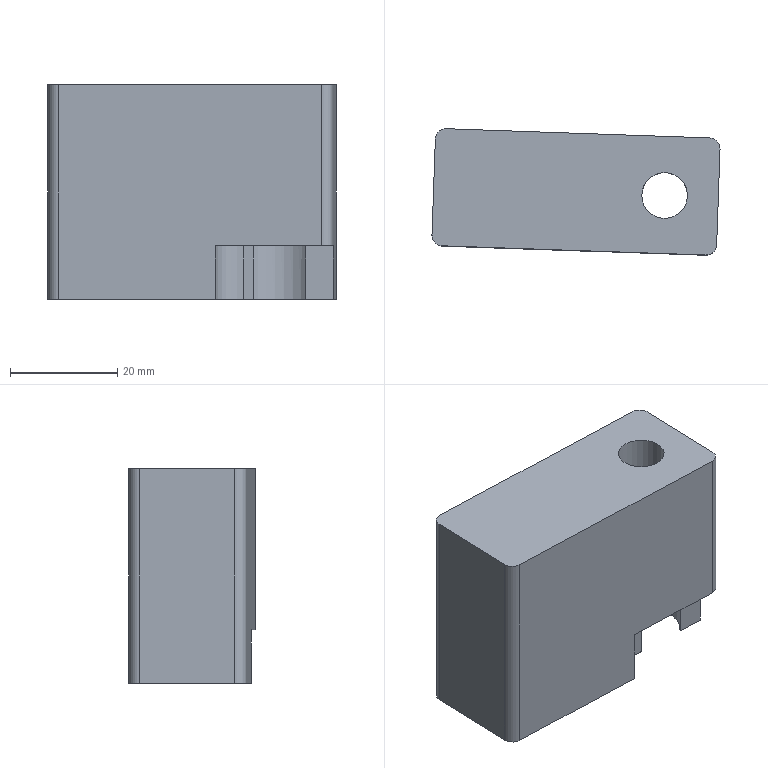Part | NX | features PS-34 2 | 1 solid | 18 faces | box 53.591 x 23.499 x 40 mm | volume 40103 mm3 | plane 11 | cylinder 7 | commonest cylinder face diameters 4 x4 8.5 x1 10 x1 14.5 x1
STEP:
#1=CARTESIAN_POINT('',(3532.617,-894.43,870.698));
#2=VERTEX_POINT('',#1);
#3=CARTESIAN_POINT('',(3530.744,-894.365,870.698));
#4=VERTEX_POINT('',#3);
#5=CARTESIAN_POINT('',(3542.677,-894.781,870.698));
#6=DIRECTION('',(-0.9994,0.0349,-0.000000001));
#7=VECTOR('',#6,1000.);
#8=LINE('',#5,#7);
#9=EDGE_CURVE('',#2,#4,#8,.T.);
#10=ORIENTED_EDGE('',*,*,#9,.T.);
#11=CARTESIAN_POINT('',(3530.744,-894.365,860.716));
#12=VERTEX_POINT('',#11);
#13=CARTESIAN_POINT('',(3530.744,-894.365,845.698));
#14=DIRECTION('',(-0.000000001,0.,1.));
#15=VECTOR('',#14,1000.);
#16=LINE('',#13,#15);
#17=EDGE_CURVE('',#4,#12,#16,.F.);
#18=ORIENTED_EDGE('',*,*,#17,.T.);
#19=CARTESIAN_POINT('',(3532.617,-894.43,860.716));
#20=VERTEX_POINT('',#19);
#21=CARTESIAN_POINT('',(3551.671,-895.095,860.716));
#22=DIRECTION('',(0.9994,-0.0349,0.));
#23=VECTOR('',#22,1000.);
#24=LINE('',#21,#23);
#25=EDGE_CURVE('',#12,#20,#24,.T.);
#26=ORIENTED_EDGE('',*,*,#25,.T.);
#27=CARTESIAN_POINT('',(3532.617,-894.43,870.698));
#28=CARTESIAN_POINT('',(3532.617,-894.43,867.371));
#29=CARTESIAN_POINT('',(3532.617,-894.43,864.044));
#30=CARTESIAN_POINT('',(3532.617,-894.43,860.716));
#31=B_SPLINE_CURVE_WITH_KNOTS('',3,(#27,#28,#29,#30),.UNSPECIFIED.,.F.,.F.,(4,4),(0.0000002,0.009982),.UNSPECIFIED.);
#32=EDGE_CURVE('',#2,#20,#31,.T.);
#33=ORIENTED_EDGE('',*,*,#32,.F.);
#34=EDGE_LOOP('',(#10,#18,#26,#33));
#35=FACE_BOUND('',#34,.T.);
#36=CARTESIAN_POINT('',(3542.677,-894.781,845.698));
#37=DIRECTION('',(0.0349,0.9994,0.));
#38=DIRECTION('',(0.9994,-0.0349,0.));
#39=AXIS2_PLACEMENT_3D('',#36,#37,#38);
#40=PLANE('',#39);
#41=ADVANCED_FACE('',(#35),#40,.F.);
#42=CARTESIAN_POINT('',(3525.557,-899.644,860.716));
#43=VERTEX_POINT('',#42);
#44=CARTESIAN_POINT('',(3525.557,-899.644,870.698));
#45=VERTEX_POINT('',#44);
#46=CARTESIAN_POINT('',(3525.557,-899.644,845.698));
#47=DIRECTION('',(-0.000000001,0.,1.));
#48=VECTOR('',#47,1000.);
#49=LINE('',#46,#48);
#50=EDGE_CURVE('',#43,#45,#49,.T.);
#51=ORIENTED_EDGE('',*,*,#50,.T.);
#52=CARTESIAN_POINT('',(3545.32,-900.334,870.698));
#53=VERTEX_POINT('',#52);
#54=CARTESIAN_POINT('',(3529.824,-899.793,870.698));
#55=DIRECTION('',(-0.9994,0.0349,-0.000000001));
#56=VECTOR('',#55,1000.);
#57=LINE('',#54,#56);
#58=EDGE_CURVE('',#53,#45,#57,.T.);
#59=ORIENTED_EDGE('',*,*,#58,.F.);
#60=CARTESIAN_POINT('',(3545.32,-900.334,900.716));
#61=VERTEX_POINT('',#60);
#62=CARTESIAN_POINT('',(3545.32,-900.334,860.716));
#63=DIRECTION('',(0.,0.,-1.));
#64=VECTOR('',#63,1000.);
#65=LINE('',#62,#64);
#66=EDGE_CURVE('',#61,#53,#65,.T.);
#67=ORIENTED_EDGE('',*,*,#66,.F.);
#68=CARTESIAN_POINT('',(3496.35,-898.624,900.716));
#69=VERTEX_POINT('',#68);
#70=CARTESIAN_POINT('',(3551.481,-900.549,900.716));
#71=DIRECTION('',(0.9994,-0.0349,0.));
#72=VECTOR('',#71,1000.);
#73=LINE('',#70,#72);
#74=EDGE_CURVE('',#69,#61,#73,.T.);
#75=ORIENTED_EDGE('',*,*,#74,.F.);
#76=CARTESIAN_POINT('',(3496.35,-898.624,860.716));
#77=VERTEX_POINT('',#76);
#78=CARTESIAN_POINT('',(3496.35,-898.624,900.716));
#79=DIRECTION('',(0.,0.,1.));
#80=VECTOR('',#79,1000.);
#81=LINE('',#78,#80);
#82=EDGE_CURVE('',#77,#69,#81,.T.);
#83=ORIENTED_EDGE('',*,*,#82,.F.);
#84=CARTESIAN_POINT('',(3551.481,-900.549,860.716));
#85=DIRECTION('',(0.9994,-0.0349,0.));
#86=VECTOR('',#85,1000.);
#87=LINE('',#84,#86);
#88=EDGE_CURVE('',#77,#43,#87,.T.);
#89=ORIENTED_EDGE('',*,*,#88,.T.);
#90=EDGE_LOOP('',(#51,#59,#67,#75,#83,#89));
#91=FACE_BOUND('',#90,.T.);
#92=CARTESIAN_POINT('',(3551.481,-900.549,950.716));
#93=DIRECTION('',(0.0349,0.9994,0.));
#94=DIRECTION('',(-0.9994,0.0349,0.));
#95=AXIS2_PLACEMENT_3D('',#92,#93,#94);
#96=PLANE('',#95);
#97=ADVANCED_FACE('',(#91),#96,.F.);
#98=CARTESIAN_POINT('',(3547.509,-894.95,870.698));
#99=VERTEX_POINT('',#98);
#100=CARTESIAN_POINT('',(3547.509,-894.95,860.716));
#101=VERTEX_POINT('',#100);
#102=CARTESIAN_POINT('',(3547.509,-894.95,860.716));
#103=DIRECTION('',(0.,0.,-1.));
#104=VECTOR('',#103,1000.);
#105=LINE('',#102,#104);
#106=EDGE_CURVE('',#99,#101,#105,.T.);
#107=ORIENTED_EDGE('',*,*,#106,.T.);
#108=CARTESIAN_POINT('',(3548.009,-880.616,860.716));
#109=VERTEX_POINT('',#108);
#110=CARTESIAN_POINT('',(3548.184,-875.619,860.716));
#111=DIRECTION('',(-0.0349,-0.9994,0.));
#112=VECTOR('',#111,1000.);
#113=LINE('',#110,#112);
#114=EDGE_CURVE('',#109,#101,#113,.T.);
#115=ORIENTED_EDGE('',*,*,#114,.F.);
#116=CARTESIAN_POINT('',(3548.009,-880.616,900.716));
#117=VERTEX_POINT('',#116);
#118=CARTESIAN_POINT('',(3548.009,-880.616,860.716));
#119=DIRECTION('',(0.,0.,-1.));
#120=VECTOR('',#119,1000.);
#121=LINE('',#118,#120);
#122=EDGE_CURVE('',#117,#109,#121,.T.);
#123=ORIENTED_EDGE('',*,*,#122,.F.);
#124=CARTESIAN_POINT('',(3547.388,-898.405,900.716));
#125=VERTEX_POINT('',#124);
#126=CARTESIAN_POINT('',(3548.184,-875.619,900.716));
#127=DIRECTION('',(-0.0349,-0.9994,0.));
#128=VECTOR('',#127,1000.);
#129=LINE('',#126,#128);
#130=EDGE_CURVE('',#117,#125,#129,.T.);
#131=ORIENTED_EDGE('',*,*,#130,.T.);
#132=CARTESIAN_POINT('',(3547.388,-898.405,870.698));
#133=VERTEX_POINT('',#132);
#134=CARTESIAN_POINT('',(3547.388,-898.405,900.716));
#135=DIRECTION('',(0.,0.,-1.));
#136=VECTOR('',#135,1000.);
#137=LINE('',#134,#136);
#138=EDGE_CURVE('',#133,#125,#137,.F.);
#139=ORIENTED_EDGE('',*,*,#138,.F.);
#140=CARTESIAN_POINT('',(3548.184,-875.619,870.698));
#141=DIRECTION('',(0.0349,0.9994,0.));
#142=VECTOR('',#141,1000.);
#143=LINE('',#140,#142);
#144=EDGE_CURVE('',#133,#99,#143,.T.);
#145=ORIENTED_EDGE('',*,*,#144,.T.);
#146=EDGE_LOOP('',(#107,#115,#123,#131,#139,#145));
#147=FACE_BOUND('',#146,.T.);
#148=CARTESIAN_POINT('',(3548.184,-875.619,860.716));
#149=DIRECTION('',(0.9994,-0.0349,0.));
#150=DIRECTION('',(-0.0349,-0.9994,0.));
#151=AXIS2_PLACEMENT_3D('',#148,#149,#150);
#152=PLANE('',#151);
#153=ADVANCED_FACE('',(#147),#152,.T.);
#154=CARTESIAN_POINT('',(3541.951,-889.261,900.716));
#155=VERTEX_POINT('',#154);
#156=CARTESIAN_POINT('',(3537.701,-889.261,900.716));
#157=DIRECTION('',(0.,0.,-1.));
#158=DIRECTION('',(1.,0.,0.));
#159=AXIS2_PLACEMENT_3D('',#156,#157,#158);
#160=CIRCLE('',#159,4.25);
#161=EDGE_CURVE('',#155,#155,#160,.T.);
#162=ORIENTED_EDGE('',*,*,#161,.T.);
#163=EDGE_LOOP('',(#162));
#164=FACE_BOUND('',#163,.T.);
#165=CARTESIAN_POINT('',(3495.042,-878.766,900.716));
#166=VERTEX_POINT('',#165);
#167=CARTESIAN_POINT('',(3494.421,-896.556,900.716));
#168=VERTEX_POINT('',#167);
#169=CARTESIAN_POINT('',(3495.216,-873.77,900.716));
#170=DIRECTION('',(-0.0349,-0.9994,0.));
#171=VECTOR('',#170,1000.);
#172=LINE('',#169,#171);
#173=EDGE_CURVE('',#166,#168,#172,.T.);
#174=ORIENTED_EDGE('',*,*,#173,.T.);
#175=CARTESIAN_POINT('',(3496.419,-896.625,900.716));
#176=DIRECTION('',(0.,0.,-1.));
#177=DIRECTION('',(1.,0.,0.));
#178=AXIS2_PLACEMENT_3D('',#175,#176,#177);
#179=CIRCLE('',#178,2.);
#180=EDGE_CURVE('',#69,#168,#179,.T.);
#181=ORIENTED_EDGE('',*,*,#180,.F.);
#182=ORIENTED_EDGE('',*,*,#74,.T.);
#183=CARTESIAN_POINT('',(3545.39,-898.335,900.716));
#184=DIRECTION('',(0.,0.,-1.));
#185=DIRECTION('',(1.,0.,0.));
#186=AXIS2_PLACEMENT_3D('',#183,#184,#185);
#187=CIRCLE('',#186,2.);
#188=EDGE_CURVE('',#125,#61,#187,.T.);
#189=ORIENTED_EDGE('',*,*,#188,.F.);
#190=ORIENTED_EDGE('',*,*,#130,.F.);
#191=CARTESIAN_POINT('',(3546.08,-878.547,900.716));
#192=VERTEX_POINT('',#191);
#193=CARTESIAN_POINT('',(3546.011,-880.546,900.716));
#194=DIRECTION('',(0.,0.,-1.));
#195=DIRECTION('',(1.,0.,0.));
#196=AXIS2_PLACEMENT_3D('',#193,#194,#195);
#197=CIRCLE('',#196,2.);
#198=EDGE_CURVE('',#192,#117,#197,.T.);
#199=ORIENTED_EDGE('',*,*,#198,.F.);
#200=CARTESIAN_POINT('',(3497.11,-876.837,900.716));
#201=VERTEX_POINT('',#200);
#202=CARTESIAN_POINT('',(3552.241,-878.762,900.716));
#203=DIRECTION('',(0.9994,-0.0349,0.));
#204=VECTOR('',#203,1000.);
#205=LINE('',#202,#204);
#206=EDGE_CURVE('',#201,#192,#205,.T.);
#207=ORIENTED_EDGE('',*,*,#206,.F.);
#208=CARTESIAN_POINT('',(3497.041,-878.836,900.716));
#209=DIRECTION('',(0.,0.,-1.));
#210=DIRECTION('',(1.,0.,0.));
#211=AXIS2_PLACEMENT_3D('',#208,#209,#210);
#212=CIRCLE('',#211,2.);
#213=EDGE_CURVE('',#166,#201,#212,.T.);
#214=ORIENTED_EDGE('',*,*,#213,.F.);
#215=EDGE_LOOP('',(#174,#181,#182,#189,#190,#199,#207,#214));
#216=FACE_BOUND('',#215,.T.);
#217=CARTESIAN_POINT('',(3552.346,-875.764,900.716));
#218=DIRECTION('',(0.,0.,1.));
#219=DIRECTION('',(1.,0.,0.));
#220=AXIS2_PLACEMENT_3D('',#217,#218,#219);
#221=PLANE('',#220);
#222=ADVANCED_FACE('',(#164,#216),#221,.T.);
#223=CARTESIAN_POINT('',(3495.042,-878.766,860.716));
#224=VERTEX_POINT('',#223);
#225=CARTESIAN_POINT('',(3494.421,-896.556,860.716));
#226=VERTEX_POINT('',#225);
#227=CARTESIAN_POINT('',(3495.216,-873.77,860.716));
#228=DIRECTION('',(-0.0349,-0.9994,0.));
#229=VECTOR('',#228,1000.);
#230=LINE('',#227,#229);
#231=EDGE_CURVE('',#224,#226,#230,.T.);
#232=ORIENTED_EDGE('',*,*,#231,.T.);
#233=CARTESIAN_POINT('',(3494.421,-896.556,860.716));
#234=DIRECTION('',(0.,0.,1.));
#235=VECTOR('',#234,1000.);
#236=LINE('',#233,#235);
#237=EDGE_CURVE('',#168,#226,#236,.F.);
#238=ORIENTED_EDGE('',*,*,#237,.F.);
#239=ORIENTED_EDGE('',*,*,#173,.F.);
#240=CARTESIAN_POINT('',(3495.042,-878.766,950.716));
#241=DIRECTION('',(0.,0.,-1.));
#242=VECTOR('',#241,1000.);
#243=LINE('',#240,#242);
#244=EDGE_CURVE('',#224,#166,#243,.F.);
#245=ORIENTED_EDGE('',*,*,#244,.F.);
#246=EDGE_LOOP('',(#232,#238,#239,#245));
#247=FACE_BOUND('',#246,.T.);
#248=CARTESIAN_POINT('',(3495.216,-873.77,950.716));
#249=DIRECTION('',(-0.9994,0.0349,0.));
#250=DIRECTION('',(0.0349,0.9994,0.));
#251=AXIS2_PLACEMENT_3D('',#248,#249,#250);
#252=PLANE('',#251);
#253=ADVANCED_FACE('',(#247),#252,.T.);
#254=ORIENTED_EDGE('',*,*,#25,.F.);
#255=CARTESIAN_POINT('',(3525.573,-899.187,860.716));
#256=VERTEX_POINT('',#255);
#257=CARTESIAN_POINT('',(3530.57,-899.361,860.716));
#258=DIRECTION('',(0.,0.,-1.));
#259=DIRECTION('',(1.,0.,0.));
#260=AXIS2_PLACEMENT_3D('',#257,#258,#259);
#261=CIRCLE('',#260,5.);
#262=EDGE_CURVE('',#12,#256,#261,.F.);
#263=ORIENTED_EDGE('',*,*,#262,.T.);
#264=CARTESIAN_POINT('',(3526.422,-874.859,860.716));
#265=DIRECTION('',(-0.0349,-0.9994,0.));
#266=VECTOR('',#265,1000.);
#267=LINE('',#264,#266);
#268=EDGE_CURVE('',#256,#43,#267,.T.);
#269=ORIENTED_EDGE('',*,*,#268,.T.);
#270=ORIENTED_EDGE('',*,*,#88,.F.);
#271=CARTESIAN_POINT('',(3496.419,-896.625,860.716));
#272=DIRECTION('',(0.,0.,-1.));
#273=DIRECTION('',(1.,0.,0.));
#274=AXIS2_PLACEMENT_3D('',#271,#272,#273);
#275=CIRCLE('',#274,2.);
#276=EDGE_CURVE('',#226,#77,#275,.F.);
#277=ORIENTED_EDGE('',*,*,#276,.F.);
#278=ORIENTED_EDGE('',*,*,#231,.F.);
#279=CARTESIAN_POINT('',(3497.11,-876.837,860.716));
#280=VERTEX_POINT('',#279);
#281=CARTESIAN_POINT('',(3497.041,-878.836,860.716));
#282=DIRECTION('',(0.,0.,-1.));
#283=DIRECTION('',(1.,0.,0.));
#284=AXIS2_PLACEMENT_3D('',#281,#282,#283);
#285=CIRCLE('',#284,2.);
#286=EDGE_CURVE('',#280,#224,#285,.F.);
#287=ORIENTED_EDGE('',*,*,#286,.F.);
#288=CARTESIAN_POINT('',(3546.08,-878.547,860.716));
#289=VERTEX_POINT('',#288);
#290=CARTESIAN_POINT('',(3552.241,-878.762,860.716));
#291=DIRECTION('',(0.9994,-0.0349,0.));
#292=VECTOR('',#291,1000.);
#293=LINE('',#290,#292);
#294=EDGE_CURVE('',#289,#280,#293,.F.);
#295=ORIENTED_EDGE('',*,*,#294,.F.);
#296=CARTESIAN_POINT('',(3546.011,-880.546,860.716));
#297=DIRECTION('',(0.,0.,-1.));
#298=DIRECTION('',(1.,0.,0.));
#299=AXIS2_PLACEMENT_3D('',#296,#297,#298);
#300=CIRCLE('',#299,2.);
#301=EDGE_CURVE('',#109,#289,#300,.F.);
#302=ORIENTED_EDGE('',*,*,#301,.F.);
#303=ORIENTED_EDGE('',*,*,#114,.T.);
#304=CARTESIAN_POINT('',(3542.413,-894.772,860.716));
#305=VERTEX_POINT('',#304);
#306=CARTESIAN_POINT('',(3551.671,-895.095,860.716));
#307=DIRECTION('',(0.9994,-0.0349,0.));
#308=VECTOR('',#307,1000.);
#309=LINE('',#306,#308);
#310=EDGE_CURVE('',#305,#101,#309,.T.);
#311=ORIENTED_EDGE('',*,*,#310,.F.);
#312=CARTESIAN_POINT('',(3537.701,-889.261,860.716));
#313=DIRECTION('',(0.,0.,-1.));
#314=DIRECTION('',(1.,0.,0.));
#315=AXIS2_PLACEMENT_3D('',#312,#313,#314);
#316=CIRCLE('',#315,7.25);
#317=EDGE_CURVE('',#20,#305,#316,.T.);
#318=ORIENTED_EDGE('',*,*,#317,.F.);
#319=EDGE_LOOP('',(#254,#263,#269,#270,#277,#278,#287,#295,#302,#303,#311,#318));
#320=FACE_BOUND('',#319,.T.);
#321=CARTESIAN_POINT('',(3552.346,-875.764,860.716));
#322=DIRECTION('',(0.,0.,1.));
#323=DIRECTION('',(1.,0.,0.));
#324=AXIS2_PLACEMENT_3D('',#321,#322,#323);
#325=PLANE('',#324);
#326=ADVANCED_FACE('',(#320),#325,.F.);
#327=ORIENTED_EDGE('',*,*,#206,.T.);
#328=CARTESIAN_POINT('',(3546.08,-878.547,880.716));
#329=DIRECTION('',(0.,0.,-1.));
#330=VECTOR('',#329,1000.);
#331=LINE('',#328,#330);
#332=EDGE_CURVE('',#289,#192,#331,.F.);
#333=ORIENTED_EDGE('',*,*,#332,.F.);
#334=ORIENTED_EDGE('',*,*,#294,.T.);
#335=CARTESIAN_POINT('',(3497.11,-876.837,880.716));
#336=DIRECTION('',(0.,0.,-1.));
#337=VECTOR('',#336,1000.);
#338=LINE('',#335,#337);
#339=EDGE_CURVE('',#201,#280,#338,.T.);
#340=ORIENTED_EDGE('',*,*,#339,.F.);
#341=EDGE_LOOP('',(#327,#333,#334,#340));
#342=FACE_BOUND('',#341,.T.);
#343=CARTESIAN_POINT('',(3514.1,-877.431,880.716));
#344=DIRECTION('',(0.0349,0.9994,0.));
#345=DIRECTION('',(0.9994,-0.0349,0.));
#346=AXIS2_PLACEMENT_3D('',#343,#344,#345);
#347=PLANE('',#346);
#348=ADVANCED_FACE('',(#342),#347,.T.);
#349=ORIENTED_EDGE('',*,*,#213,.T.);
#350=ORIENTED_EDGE('',*,*,#339,.T.);
#351=ORIENTED_EDGE('',*,*,#286,.T.);
#352=ORIENTED_EDGE('',*,*,#244,.T.);
#353=EDGE_LOOP('',(#349,#350,#351,#352));
#354=FACE_BOUND('',#353,.T.);
#355=CARTESIAN_POINT('',(3497.041,-878.836,880.716));
#356=DIRECTION('',(0.,0.,-1.));
#357=DIRECTION('',(-1.,0.,0.));
#358=AXIS2_PLACEMENT_3D('',#355,#356,#357);
#359=CYLINDRICAL_SURFACE('',#358,2.);
#360=ADVANCED_FACE('',(#354),#359,.T.);
#361=ORIENTED_EDGE('',*,*,#198,.T.);
#362=ORIENTED_EDGE('',*,*,#122,.T.);
#363=ORIENTED_EDGE('',*,*,#301,.T.);
#364=ORIENTED_EDGE('',*,*,#332,.T.);
#365=EDGE_LOOP('',(#361,#362,#363,#364));
#366=FACE_BOUND('',#365,.T.);
#367=CARTESIAN_POINT('',(3546.011,-880.546,860.716));
#368=DIRECTION('',(0.,0.,-1.));
#369=DIRECTION('',(-1.,0.,0.));
#370=AXIS2_PLACEMENT_3D('',#367,#368,#369);
#371=CYLINDRICAL_SURFACE('',#370,2.);
#372=ADVANCED_FACE('',(#366),#371,.T.);
#373=CARTESIAN_POINT('',(3545.39,-898.335,870.698));
#374=DIRECTION('',(0.000000001,0.,-1.));
#375=DIRECTION('',(1.,0.,0.000000001));
#376=AXIS2_PLACEMENT_3D('',#373,#374,#375);
#377=CIRCLE('',#376,2.);
#378=EDGE_CURVE('',#53,#133,#377,.F.);
#379=ORIENTED_EDGE('',*,*,#378,.T.);
#380=ORIENTED_EDGE('',*,*,#138,.T.);
#381=ORIENTED_EDGE('',*,*,#188,.T.);
#382=ORIENTED_EDGE('',*,*,#66,.T.);
#383=EDGE_LOOP('',(#379,#380,#381,#382));
#384=FACE_BOUND('',#383,.T.);
#385=CARTESIAN_POINT('',(3545.39,-898.335,950.716));
#386=DIRECTION('',(0.,0.,1.));
#387=DIRECTION('',(1.,0.,0.));
#388=AXIS2_PLACEMENT_3D('',#385,#386,#387);
#389=CYLINDRICAL_SURFACE('',#388,2.);
#390=ADVANCED_FACE('',(#384),#389,.T.);
#391=ORIENTED_EDGE('',*,*,#276,.T.);
#392=ORIENTED_EDGE('',*,*,#82,.T.);
#393=ORIENTED_EDGE('',*,*,#180,.T.);
#394=ORIENTED_EDGE('',*,*,#237,.T.);
#395=EDGE_LOOP('',(#391,#392,#393,#394));
#396=FACE_BOUND('',#395,.T.);
#397=CARTESIAN_POINT('',(3496.419,-896.625,950.716));
#398=DIRECTION('',(0.,0.,-1.));
#399=DIRECTION('',(-1.,0.,0.));
#400=AXIS2_PLACEMENT_3D('',#397,#398,#399);
#401=CYLINDRICAL_SURFACE('',#400,2.);
#402=ADVANCED_FACE('',(#396),#401,.T.);
#403=ORIENTED_EDGE('',*,*,#262,.F.);
#404=ORIENTED_EDGE('',*,*,#17,.F.);
#405=CARTESIAN_POINT('',(3525.573,-899.187,870.698));
#406=VERTEX_POINT('',#405);
#407=CARTESIAN_POINT('',(3530.57,-899.361,870.698));
#408=DIRECTION('',(0.000000001,0.,-1.));
#409=DIRECTION('',(1.,0.,0.000000001));
#410=AXIS2_PLACEMENT_3D('',#407,#408,#409);
#411=CIRCLE('',#410,5.);
#412=EDGE_CURVE('',#406,#4,#411,.T.);
#413=ORIENTED_EDGE('',*,*,#412,.F.);
#414=CARTESIAN_POINT('',(3525.573,-899.187,845.698));
#415=DIRECTION('',(-0.000000001,0.,1.));
#416=VECTOR('',#415,1000.);
#417=LINE('',#414,#416);
#418=EDGE_CURVE('',#406,#256,#417,.F.);
#419=ORIENTED_EDGE('',*,*,#418,.T.);
#420=EDGE_LOOP('',(#403,#404,#413,#419));
#421=FACE_BOUND('',#420,.T.);
#422=CARTESIAN_POINT('',(3530.57,-899.361,845.698));
#423=DIRECTION('',(-0.000000001,0.,1.));
#424=DIRECTION('',(1.,0.,0.000000001));
#425=AXIS2_PLACEMENT_3D('',#422,#423,#424);
#426=CYLINDRICAL_SURFACE('',#425,5.);
#427=ADVANCED_FACE('',(#421),#426,.F.);
#428=ORIENTED_EDGE('',*,*,#268,.F.);
#429=ORIENTED_EDGE('',*,*,#418,.F.);
#430=CARTESIAN_POINT('',(3525.258,-908.206,870.698));
#431=DIRECTION('',(0.0349,0.9994,0.));
#432=VECTOR('',#431,1000.);
#433=LINE('',#430,#432);
#434=EDGE_CURVE('',#45,#406,#433,.T.);
#435=ORIENTED_EDGE('',*,*,#434,.F.);
#436=ORIENTED_EDGE('',*,*,#50,.F.);
#437=EDGE_LOOP('',(#428,#429,#435,#436));
#438=FACE_BOUND('',#437,.T.);
#439=CARTESIAN_POINT('',(3525.258,-908.206,845.698));
#440=DIRECTION('',(0.9994,-0.0349,0.000000001));
#441=DIRECTION('',(-0.0349,-0.9994,0.));
#442=AXIS2_PLACEMENT_3D('',#439,#440,#441);
#443=PLANE('',#442);
#444=ADVANCED_FACE('',(#438),#443,.T.);
#445=ORIENTED_EDGE('',*,*,#310,.T.);
#446=ORIENTED_EDGE('',*,*,#106,.F.);
#447=CARTESIAN_POINT('',(3542.413,-894.772,870.698));
#448=VERTEX_POINT('',#447);
#449=CARTESIAN_POINT('',(3542.677,-894.781,870.698));
#450=DIRECTION('',(-0.9994,0.0349,-0.000000001));
#451=VECTOR('',#450,1000.);
#452=LINE('',#449,#451);
#453=EDGE_CURVE('',#99,#448,#452,.T.);
#454=ORIENTED_EDGE('',*,*,#453,.T.);
#455=CARTESIAN_POINT('',(3542.413,-894.772,860.716));
#456=CARTESIAN_POINT('',(3542.413,-894.772,864.044));
#457=CARTESIAN_POINT('',(3542.413,-894.772,867.371));
#458=CARTESIAN_POINT('',(3542.413,-894.772,870.698));
#459=B_SPLINE_CURVE_WITH_KNOTS('',3,(#455,#456,#457,#458),.UNSPECIFIED.,.F.,.F.,(4,4),(0.0000002,0.009982),.UNSPECIFIED.);
#460=EDGE_CURVE('',#305,#448,#459,.T.);
#461=ORIENTED_EDGE('',*,*,#460,.F.);
#462=EDGE_LOOP('',(#445,#446,#454,#461));
#463=FACE_BOUND('',#462,.T.);
#464=CARTESIAN_POINT('',(3542.677,-894.781,845.698));
#465=DIRECTION('',(0.0349,0.9994,0.));
#466=DIRECTION('',(0.9994,-0.0349,0.));
#467=AXIS2_PLACEMENT_3D('',#464,#465,#466);
#468=PLANE('',#467);
#469=ADVANCED_FACE('',(#463),#468,.F.);
#470=ORIENTED_EDGE('',*,*,#453,.F.);
#471=ORIENTED_EDGE('',*,*,#144,.F.);
#472=ORIENTED_EDGE('',*,*,#378,.F.);
#473=ORIENTED_EDGE('',*,*,#58,.T.);
#474=ORIENTED_EDGE('',*,*,#434,.T.);
#475=ORIENTED_EDGE('',*,*,#412,.T.);
#476=ORIENTED_EDGE('',*,*,#9,.F.);
#477=CARTESIAN_POINT('',(3537.701,-889.261,870.698));
#478=DIRECTION('',(0.000000001,0.,-1.));
#479=DIRECTION('',(1.,0.,0.000000001));
#480=AXIS2_PLACEMENT_3D('',#477,#478,#479);
#481=CIRCLE('',#480,7.25);
#482=EDGE_CURVE('',#448,#2,#481,.T.);
#483=ORIENTED_EDGE('',*,*,#482,.F.);
#484=EDGE_LOOP('',(#470,#471,#472,#473,#474,#475,#476,#483));
#485=FACE_BOUND('',#484,.T.);
#486=CARTESIAN_POINT('',(3529.525,-908.355,870.698));
#487=DIRECTION('',(-0.000000001,0.,1.));
#488=DIRECTION('',(1.,0.,0.000000001));
#489=AXIS2_PLACEMENT_3D('',#486,#487,#488);
#490=PLANE('',#489);
#491=ADVANCED_FACE('',(#485),#490,.F.);
#492=CARTESIAN_POINT('',(3530.451,-889.261,885.716));
#493=VERTEX_POINT('',#492);
#494=CARTESIAN_POINT('',(3537.701,-889.261,885.716));
#495=DIRECTION('',(0.,0.,1.));
#496=DIRECTION('',(-1.,0.,0.));
#497=AXIS2_PLACEMENT_3D('',#494,#495,#496);
#498=CIRCLE('',#497,7.25);
#499=EDGE_CURVE('',#493,#493,#498,.F.);
#500=ORIENTED_EDGE('',*,*,#499,.F.);
#501=EDGE_LOOP('',(#500));
#502=FACE_BOUND('',#501,.T.);
#503=ORIENTED_EDGE('',*,*,#32,.T.);
#504=ORIENTED_EDGE('',*,*,#317,.T.);
#505=ORIENTED_EDGE('',*,*,#460,.T.);
#506=ORIENTED_EDGE('',*,*,#482,.T.);
#507=EDGE_LOOP('',(#503,#504,#505,#506));
#508=FACE_BOUND('',#507,.T.);
#509=CARTESIAN_POINT('',(3537.701,-889.261,875.716));
#510=DIRECTION('',(0.,0.,-1.));
#511=DIRECTION('',(-1.,0.,0.));
#512=AXIS2_PLACEMENT_3D('',#509,#510,#511);
#513=CYLINDRICAL_SURFACE('',#512,7.25);
#514=ADVANCED_FACE('',(#502,#508),#513,.F.);
#515=ORIENTED_EDGE('',*,*,#161,.F.);
#516=EDGE_LOOP('',(#515));
#517=FACE_BOUND('',#516,.T.);
#518=CARTESIAN_POINT('',(3533.451,-889.261,885.716));
#519=VERTEX_POINT('',#518);
#520=CARTESIAN_POINT('',(3537.701,-889.261,885.716));
#521=DIRECTION('',(0.,0.,1.));
#522=DIRECTION('',(-1.,0.,0.));
#523=AXIS2_PLACEMENT_3D('',#520,#521,#522);
#524=CIRCLE('',#523,4.25);
#525=EDGE_CURVE('',#519,#519,#524,.T.);
#526=ORIENTED_EDGE('',*,*,#525,.F.);
#527=EDGE_LOOP('',(#526));
#528=FACE_BOUND('',#527,.T.);
#529=CARTESIAN_POINT('',(3537.701,-889.261,901.716));
#530=DIRECTION('',(0.,0.,-1.));
#531=DIRECTION('',(-1.,0.,0.));
#532=AXIS2_PLACEMENT_3D('',#529,#530,#531);
#533=CYLINDRICAL_SURFACE('',#532,4.25);
#534=ADVANCED_FACE('',(#517,#528),#533,.F.);
#535=ORIENTED_EDGE('',*,*,#525,.T.);
#536=EDGE_LOOP('',(#535));
#537=FACE_BOUND('',#536,.T.);
#538=ORIENTED_EDGE('',*,*,#499,.T.);
#539=EDGE_LOOP('',(#538));
#540=FACE_BOUND('',#539,.T.);
#541=CARTESIAN_POINT('',(3537.701,-889.261,885.716));
#542=DIRECTION('',(0.,0.,-1.));
#543=DIRECTION('',(-1.,0.,0.));
#544=AXIS2_PLACEMENT_3D('',#541,#542,#543);
#545=PLANE('',#544);
#546=ADVANCED_FACE('',(#537,#540),#545,.T.);
#547=CLOSED_SHELL('',(#41,#97,#153,#222,#253,#326,#348,#360,#372,#390,#402,#427,#444,#469,#491,#514,#534,#546));
#548=MANIFOLD_SOLID_BREP('',#547);
#549=(LENGTH_UNIT()NAMED_UNIT(*)SI_UNIT(.MILLI.,.METRE.));
#550=UNCERTAINTY_MEASURE_WITH_UNIT(LENGTH_MEASURE(0.0508),#549,'','');
#551=(NAMED_UNIT(*)PLANE_ANGLE_UNIT()SI_UNIT($,.RADIAN.));
#552=(NAMED_UNIT(*)SI_UNIT($,.STERADIAN.)SOLID_ANGLE_UNIT());
#553=(GEOMETRIC_REPRESENTATION_CONTEXT(3)GLOBAL_UNCERTAINTY_ASSIGNED_CONTEXT((#550))GLOBAL_UNIT_ASSIGNED_CONTEXT((#549,#551,#552))REPRESENTATION_CONTEXT('',''));
#554=ADVANCED_BREP_SHAPE_REPRESENTATION('',(#548),#553);